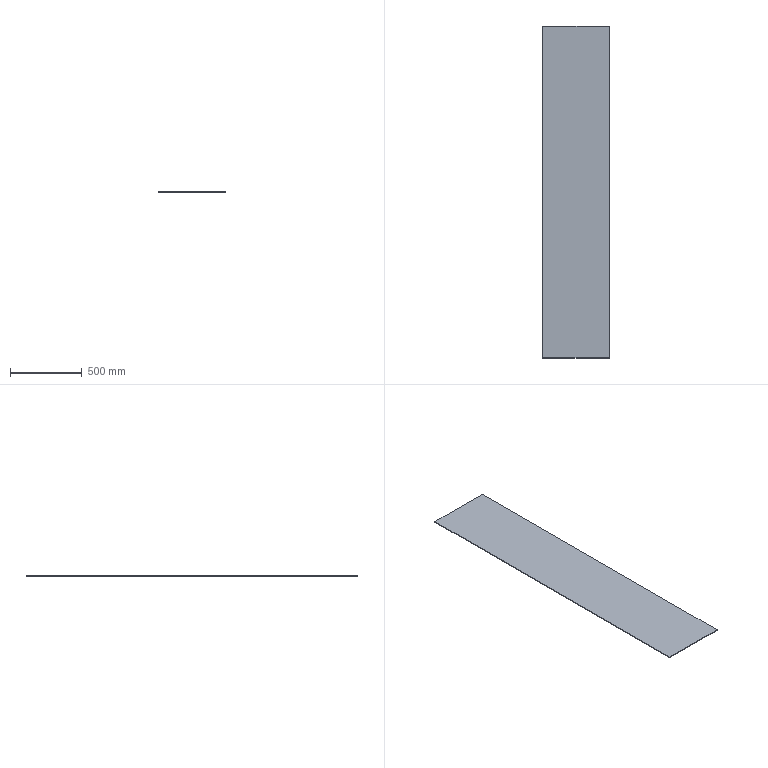Part | SolidWorks | features Extrusion 1, HoleWzd 1 | 1 solid | 6 faces | box 466 x 2310 x 5 mm | volume 5382300 mm3 | plane 6
STEP:
#1=CARTESIAN_POINT('',(233.,-1155.,0.));
#2=VERTEX_POINT('',#1);
#3=CARTESIAN_POINT('',(233.,1155.,0.));
#4=VERTEX_POINT('',#3);
#5=CARTESIAN_POINT('',(233.,1155.,0.));
#6=DIRECTION('',(0.,1.,0.));
#7=VECTOR('',#6,1000.);
#8=LINE('',#5,#7);
#9=EDGE_CURVE('',#2,#4,#8,.T.);
#10=ORIENTED_EDGE('',*,*,#9,.T.);
#11=CARTESIAN_POINT('',(233.,1155.,5.));
#12=VERTEX_POINT('',#11);
#13=CARTESIAN_POINT('',(233.,1155.,5.));
#14=DIRECTION('',(0.,0.,-1.));
#15=VECTOR('',#14,1000.);
#16=LINE('',#13,#15);
#17=EDGE_CURVE('',#12,#4,#16,.T.);
#18=ORIENTED_EDGE('',*,*,#17,.F.);
#19=CARTESIAN_POINT('',(233.,-1155.,5.));
#20=VERTEX_POINT('',#19);
#21=CARTESIAN_POINT('',(233.,1155.,5.));
#22=DIRECTION('',(0.,1.,0.));
#23=VECTOR('',#22,1000.);
#24=LINE('',#21,#23);
#25=EDGE_CURVE('',#20,#12,#24,.T.);
#26=ORIENTED_EDGE('',*,*,#25,.F.);
#27=CARTESIAN_POINT('',(233.,-1155.,5.));
#28=DIRECTION('',(0.,0.,-1.));
#29=VECTOR('',#28,1000.);
#30=LINE('',#27,#29);
#31=EDGE_CURVE('',#20,#2,#30,.T.);
#32=ORIENTED_EDGE('',*,*,#31,.T.);
#33=EDGE_LOOP('',(#10,#18,#26,#32));
#34=FACE_OUTER_BOUND('',#33,.T.);
#35=CARTESIAN_POINT('',(233.,1155.,5.));
#36=DIRECTION('',(-1.,0.,0.));
#37=DIRECTION('',(0.,-1.,0.));
#38=AXIS2_PLACEMENT_3D('',#35,#36,#37);
#39=PLANE('',#38);
#40=ADVANCED_FACE('',(#34),#39,.F.);
#41=CARTESIAN_POINT('',(-233.,1155.,0.));
#42=VERTEX_POINT('',#41);
#43=CARTESIAN_POINT('',(-233.,1155.,0.));
#44=DIRECTION('',(-1.,0.,0.));
#45=VECTOR('',#44,1000.);
#46=LINE('',#43,#45);
#47=EDGE_CURVE('',#4,#42,#46,.T.);
#48=ORIENTED_EDGE('',*,*,#47,.T.);
#49=CARTESIAN_POINT('',(-233.,1155.,5.));
#50=VERTEX_POINT('',#49);
#51=CARTESIAN_POINT('',(-233.,1155.,5.));
#52=DIRECTION('',(0.,0.,-1.));
#53=VECTOR('',#52,1000.);
#54=LINE('',#51,#53);
#55=EDGE_CURVE('',#50,#42,#54,.T.);
#56=ORIENTED_EDGE('',*,*,#55,.F.);
#57=CARTESIAN_POINT('',(-233.,1155.,5.));
#58=DIRECTION('',(-1.,0.,0.));
#59=VECTOR('',#58,1000.);
#60=LINE('',#57,#59);
#61=EDGE_CURVE('',#12,#50,#60,.T.);
#62=ORIENTED_EDGE('',*,*,#61,.F.);
#63=ORIENTED_EDGE('',*,*,#17,.T.);
#64=EDGE_LOOP('',(#48,#56,#62,#63));
#65=FACE_OUTER_BOUND('',#64,.T.);
#66=CARTESIAN_POINT('',(-233.,1155.,5.));
#67=DIRECTION('',(0.,-1.,0.));
#68=DIRECTION('',(0.,0.,-1.));
#69=AXIS2_PLACEMENT_3D('',#66,#67,#68);
#70=PLANE('',#69);
#71=ADVANCED_FACE('',(#65),#70,.F.);
#72=CARTESIAN_POINT('',(-233.,-1155.,0.));
#73=VERTEX_POINT('',#72);
#74=CARTESIAN_POINT('',(-233.,1155.,0.));
#75=DIRECTION('',(0.,-1.,0.));
#76=VECTOR('',#75,1000.);
#77=LINE('',#74,#76);
#78=EDGE_CURVE('',#42,#73,#77,.T.);
#79=ORIENTED_EDGE('',*,*,#78,.T.);
#80=CARTESIAN_POINT('',(-233.,-1155.,5.));
#81=VERTEX_POINT('',#80);
#82=CARTESIAN_POINT('',(-233.,-1155.,5.));
#83=DIRECTION('',(0.,0.,-1.));
#84=VECTOR('',#83,1000.);
#85=LINE('',#82,#84);
#86=EDGE_CURVE('',#81,#73,#85,.T.);
#87=ORIENTED_EDGE('',*,*,#86,.F.);
#88=CARTESIAN_POINT('',(-233.,1155.,5.));
#89=DIRECTION('',(0.,-1.,0.));
#90=VECTOR('',#89,1000.);
#91=LINE('',#88,#90);
#92=EDGE_CURVE('',#50,#81,#91,.T.);
#93=ORIENTED_EDGE('',*,*,#92,.F.);
#94=ORIENTED_EDGE('',*,*,#55,.T.);
#95=EDGE_LOOP('',(#79,#87,#93,#94));
#96=FACE_OUTER_BOUND('',#95,.T.);
#97=CARTESIAN_POINT('',(-233.,1155.,5.));
#98=DIRECTION('',(1.,0.,0.));
#99=DIRECTION('',(0.,1.,0.));
#100=AXIS2_PLACEMENT_3D('',#97,#98,#99);
#101=PLANE('',#100);
#102=ADVANCED_FACE('',(#96),#101,.F.);
#103=CARTESIAN_POINT('',(-233.,-1155.,0.));
#104=DIRECTION('',(1.,0.,0.));
#105=VECTOR('',#104,1000.);
#106=LINE('',#103,#105);
#107=EDGE_CURVE('',#73,#2,#106,.T.);
#108=ORIENTED_EDGE('',*,*,#107,.T.);
#109=ORIENTED_EDGE('',*,*,#31,.F.);
#110=CARTESIAN_POINT('',(-233.,-1155.,5.));
#111=DIRECTION('',(1.,0.,0.));
#112=VECTOR('',#111,1000.);
#113=LINE('',#110,#112);
#114=EDGE_CURVE('',#81,#20,#113,.T.);
#115=ORIENTED_EDGE('',*,*,#114,.F.);
#116=ORIENTED_EDGE('',*,*,#86,.T.);
#117=EDGE_LOOP('',(#108,#109,#115,#116));
#118=FACE_OUTER_BOUND('',#117,.T.);
#119=CARTESIAN_POINT('',(-233.,-1155.,5.));
#120=DIRECTION('',(0.,1.,0.));
#121=DIRECTION('',(0.,0.,1.));
#122=AXIS2_PLACEMENT_3D('',#119,#120,#121);
#123=PLANE('',#122);
#124=ADVANCED_FACE('',(#118),#123,.F.);
#125=ORIENTED_EDGE('',*,*,#25,.T.);
#126=ORIENTED_EDGE('',*,*,#61,.T.);
#127=ORIENTED_EDGE('',*,*,#92,.T.);
#128=ORIENTED_EDGE('',*,*,#114,.T.);
#129=EDGE_LOOP('',(#125,#126,#127,#128));
#130=FACE_OUTER_BOUND('',#129,.T.);
#131=CARTESIAN_POINT('',(0.,0.,5.));
#132=DIRECTION('',(0.,0.,1.));
#133=DIRECTION('',(1.,0.,0.));
#134=AXIS2_PLACEMENT_3D('',#131,#132,#133);
#135=PLANE('',#134);
#136=ADVANCED_FACE('',(#130),#135,.T.);
#137=ORIENTED_EDGE('',*,*,#9,.F.);
#138=ORIENTED_EDGE('',*,*,#107,.F.);
#139=ORIENTED_EDGE('',*,*,#78,.F.);
#140=ORIENTED_EDGE('',*,*,#47,.F.);
#141=EDGE_LOOP('',(#137,#138,#139,#140));
#142=FACE_OUTER_BOUND('',#141,.T.);
#143=CARTESIAN_POINT('',(0.,0.,0.));
#144=DIRECTION('',(0.,0.,1.));
#145=DIRECTION('',(1.,0.,0.));
#146=AXIS2_PLACEMENT_3D('',#143,#144,#145);
#147=PLANE('',#146);
#148=ADVANCED_FACE('',(#142),#147,.F.);
#149=CLOSED_SHELL('',(#40,#71,#102,#124,#136,#148));
#150=MANIFOLD_SOLID_BREP('',#149);
#151=CARTESIAN_POINT('',(0.,0.,0.));
#152=DIRECTION('',(0.,0.,1.));
#153=DIRECTION('',(1.,0.,0.));
#154=AXIS2_PLACEMENT_3D('',#151,#152,#153);
#155=(LENGTH_UNIT()NAMED_UNIT(*)SI_UNIT(.MILLI.,.METRE.));
#156=UNCERTAINTY_MEASURE_WITH_UNIT(LENGTH_MEASURE(0.00001),#155,'','');
#157=(NAMED_UNIT(*)PLANE_ANGLE_UNIT()SI_UNIT($,.RADIAN.));
#158=(NAMED_UNIT(*)SI_UNIT($,.STERADIAN.)SOLID_ANGLE_UNIT());
#159=(GEOMETRIC_REPRESENTATION_CONTEXT(3)GLOBAL_UNCERTAINTY_ASSIGNED_CONTEXT((#156))GLOBAL_UNIT_ASSIGNED_CONTEXT((#155,#157,#158))REPRESENTATION_CONTEXT('',''));
#160=ADVANCED_BREP_SHAPE_REPRESENTATION('',(#150,#154),#159);